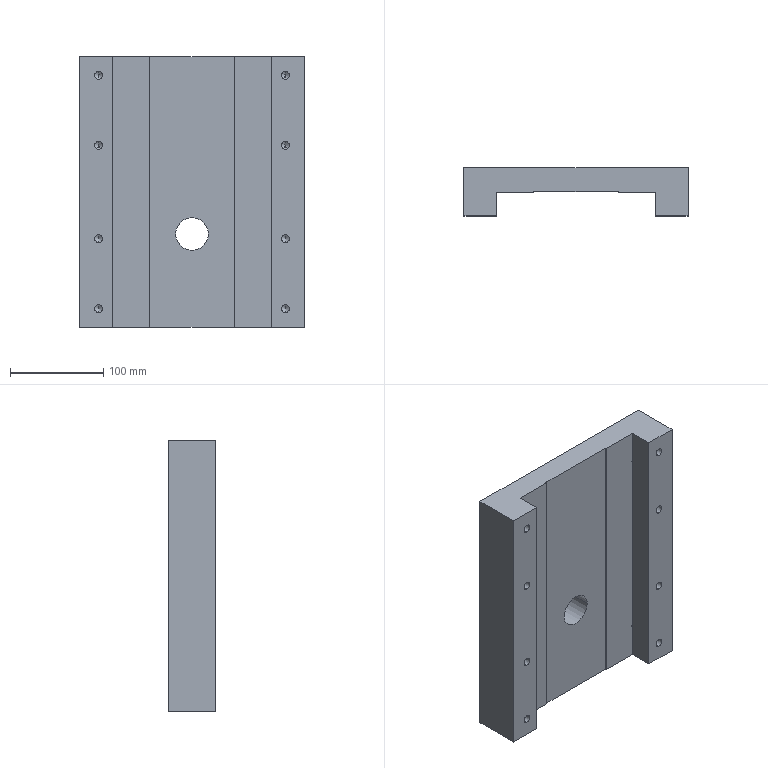Part | SolidWorks | features HoleWzd 2, Extrusion 1, ICE 1 | 1 solid | 64 faces | box 240 x 51 x 290 mm | volume 2244437 mm3 | cylinder 26 | cone 24 | plane 14 | commonest cylinder face diameters 8.5 x16 10.2 x8 35 x2